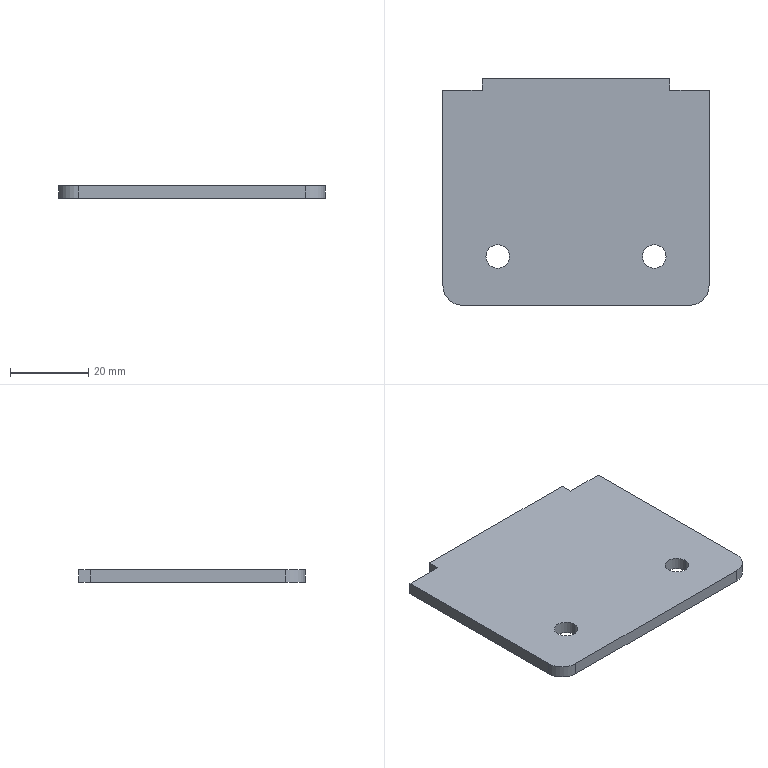Part | SolidWorks | features FlatPattern 1, SMBaseFlange 1, SheetMetal 1 | 1 solid | 16 faces | box 68 x 57.9 x 3.2 mm | volume 12192 mm3 | plane 10 | cylinder 6 | commonest cylinder face diameters 6 x4 10 x2
STEP:
#1=CARTESIAN_POINT('',(-23.,0.,3.2));
#2=VERTEX_POINT('',#1);
#3=CARTESIAN_POINT('',(-17.,0.,3.2));
#4=VERTEX_POINT('',#3);
#5=CARTESIAN_POINT('',(-20.,0.,3.2));
#6=DIRECTION('',(0.,0.,1.));
#7=DIRECTION('',(1.,0.,0.));
#8=AXIS2_PLACEMENT_3D('',#5,#6,#7);
#9=CIRCLE('',#8,3.);
#10=EDGE_CURVE('',#2,#4,#9,.T.);
#11=ORIENTED_EDGE('',*,*,#10,.T.);
#12=CARTESIAN_POINT('',(-17.,0.,0.));
#13=VERTEX_POINT('',#12);
#14=CARTESIAN_POINT('',(-17.,0.,3.2));
#15=DIRECTION('',(0.,0.,-1.));
#16=VECTOR('',#15,1000.);
#17=LINE('',#14,#16);
#18=EDGE_CURVE('',#4,#13,#17,.T.);
#19=ORIENTED_EDGE('',*,*,#18,.T.);
#20=CARTESIAN_POINT('',(-23.,0.,0.));
#21=VERTEX_POINT('',#20);
#22=CARTESIAN_POINT('',(-20.,0.,0.));
#23=DIRECTION('',(0.,0.,1.));
#24=DIRECTION('',(1.,0.,0.));
#25=AXIS2_PLACEMENT_3D('',#22,#23,#24);
#26=CIRCLE('',#25,3.);
#27=EDGE_CURVE('',#21,#13,#26,.T.);
#28=ORIENTED_EDGE('',*,*,#27,.F.);
#29=CARTESIAN_POINT('',(-23.,0.,3.2));
#30=DIRECTION('',(0.,0.,-1.));
#31=VECTOR('',#30,1000.);
#32=LINE('',#29,#31);
#33=EDGE_CURVE('',#2,#21,#32,.T.);
#34=ORIENTED_EDGE('',*,*,#33,.F.);
#35=EDGE_LOOP('',(#11,#19,#28,#34));
#36=FACE_OUTER_BOUND('',#35,.T.);
#37=CARTESIAN_POINT('',(-20.,0.,3.2));
#38=DIRECTION('',(0.,0.,-1.));
#39=DIRECTION('',(-1.,0.,0.));
#40=AXIS2_PLACEMENT_3D('',#37,#38,#39);
#41=CYLINDRICAL_SURFACE('',#40,3.);
#42=ADVANCED_FACE('',(#36),#41,.F.);
#43=CARTESIAN_POINT('',(17.,0.,3.2));
#44=VERTEX_POINT('',#43);
#45=CARTESIAN_POINT('',(23.,0.,3.2));
#46=VERTEX_POINT('',#45);
#47=CARTESIAN_POINT('',(20.,0.,3.2));
#48=DIRECTION('',(0.,0.,1.));
#49=DIRECTION('',(1.,0.,0.));
#50=AXIS2_PLACEMENT_3D('',#47,#48,#49);
#51=CIRCLE('',#50,3.);
#52=EDGE_CURVE('',#44,#46,#51,.T.);
#53=ORIENTED_EDGE('',*,*,#52,.T.);
#54=CARTESIAN_POINT('',(23.,0.,0.));
#55=VERTEX_POINT('',#54);
#56=CARTESIAN_POINT('',(23.,0.,3.2));
#57=DIRECTION('',(0.,0.,-1.));
#58=VECTOR('',#57,1000.);
#59=LINE('',#56,#58);
#60=EDGE_CURVE('',#46,#55,#59,.T.);
#61=ORIENTED_EDGE('',*,*,#60,.T.);
#62=CARTESIAN_POINT('',(17.,0.,0.));
#63=VERTEX_POINT('',#62);
#64=CARTESIAN_POINT('',(20.,0.,0.));
#65=DIRECTION('',(0.,0.,1.));
#66=DIRECTION('',(1.,0.,0.));
#67=AXIS2_PLACEMENT_3D('',#64,#65,#66);
#68=CIRCLE('',#67,3.);
#69=EDGE_CURVE('',#63,#55,#68,.T.);
#70=ORIENTED_EDGE('',*,*,#69,.F.);
#71=CARTESIAN_POINT('',(17.,0.,3.2));
#72=DIRECTION('',(0.,0.,-1.));
#73=VECTOR('',#72,1000.);
#74=LINE('',#71,#73);
#75=EDGE_CURVE('',#44,#63,#74,.T.);
#76=ORIENTED_EDGE('',*,*,#75,.F.);
#77=EDGE_LOOP('',(#53,#61,#70,#76));
#78=FACE_OUTER_BOUND('',#77,.T.);
#79=CARTESIAN_POINT('',(20.,0.,3.2));
#80=DIRECTION('',(0.,0.,-1.));
#81=DIRECTION('',(-1.,0.,0.));
#82=AXIS2_PLACEMENT_3D('',#79,#80,#81);
#83=CYLINDRICAL_SURFACE('',#82,3.);
#84=ADVANCED_FACE('',(#78),#83,.F.);
#85=CARTESIAN_POINT('',(34.,-7.5,3.2));
#86=VERTEX_POINT('',#85);
#87=CARTESIAN_POINT('',(34.,42.4,3.2));
#88=VERTEX_POINT('',#87);
#89=CARTESIAN_POINT('',(34.,0.,3.2));
#90=DIRECTION('',(0.,1.,0.));
#91=VECTOR('',#90,1000.);
#92=LINE('',#89,#91);
#93=EDGE_CURVE('',#86,#88,#92,.T.);
#94=ORIENTED_EDGE('',*,*,#93,.T.);
#95=CARTESIAN_POINT('',(24.,42.4,3.2));
#96=VERTEX_POINT('',#95);
#97=CARTESIAN_POINT('',(34.,42.4,3.2));
#98=DIRECTION('',(-1.,0.,0.));
#99=VECTOR('',#98,1000.);
#100=LINE('',#97,#99);
#101=EDGE_CURVE('',#88,#96,#100,.T.);
#102=ORIENTED_EDGE('',*,*,#101,.T.);
#103=CARTESIAN_POINT('',(24.,45.4,3.2));
#104=VERTEX_POINT('',#103);
#105=CARTESIAN_POINT('',(24.,42.4,3.2));
#106=DIRECTION('',(0.,1.,0.));
#107=VECTOR('',#106,1000.);
#108=LINE('',#105,#107);
#109=EDGE_CURVE('',#96,#104,#108,.T.);
#110=ORIENTED_EDGE('',*,*,#109,.T.);
#111=CARTESIAN_POINT('',(-24.,45.4,3.2));
#112=VERTEX_POINT('',#111);
#113=CARTESIAN_POINT('',(24.,45.4,3.2));
#114=DIRECTION('',(-1.,0.,0.));
#115=VECTOR('',#114,1000.);
#116=LINE('',#113,#115);
#117=EDGE_CURVE('',#104,#112,#116,.T.);
#118=ORIENTED_EDGE('',*,*,#117,.T.);
#119=CARTESIAN_POINT('',(-24.,42.4,3.2));
#120=VERTEX_POINT('',#119);
#121=CARTESIAN_POINT('',(-24.,45.4,3.2));
#122=DIRECTION('',(0.,-1.,0.));
#123=VECTOR('',#122,1000.);
#124=LINE('',#121,#123);
#125=EDGE_CURVE('',#112,#120,#124,.T.);
#126=ORIENTED_EDGE('',*,*,#125,.T.);
#127=CARTESIAN_POINT('',(-34.,42.4,3.2));
#128=VERTEX_POINT('',#127);
#129=CARTESIAN_POINT('',(-24.,42.4,3.2));
#130=DIRECTION('',(-1.,0.,0.));
#131=VECTOR('',#130,1000.);
#132=LINE('',#129,#131);
#133=EDGE_CURVE('',#120,#128,#132,.T.);
#134=ORIENTED_EDGE('',*,*,#133,.T.);
#135=CARTESIAN_POINT('',(-34.,-7.5,3.2));
#136=VERTEX_POINT('',#135);
#137=CARTESIAN_POINT('',(-34.,42.4,3.2));
#138=DIRECTION('',(0.,-1.,0.));
#139=VECTOR('',#138,1000.);
#140=LINE('',#137,#139);
#141=EDGE_CURVE('',#128,#136,#140,.T.);
#142=ORIENTED_EDGE('',*,*,#141,.T.);
#143=CARTESIAN_POINT('',(-29.,-12.5,3.2));
#144=VERTEX_POINT('',#143);
#145=CARTESIAN_POINT('',(-29.,-7.5,3.2));
#146=DIRECTION('',(0.,0.,1.));
#147=DIRECTION('',(-1.,0.,0.));
#148=AXIS2_PLACEMENT_3D('',#145,#146,#147);
#149=CIRCLE('',#148,5.);
#150=EDGE_CURVE('',#136,#144,#149,.T.);
#151=ORIENTED_EDGE('',*,*,#150,.T.);
#152=CARTESIAN_POINT('',(29.,-12.5,3.2));
#153=VERTEX_POINT('',#152);
#154=CARTESIAN_POINT('',(29.,-12.5,3.2));
#155=DIRECTION('',(1.,0.,0.));
#156=VECTOR('',#155,1000.);
#157=LINE('',#154,#156);
#158=EDGE_CURVE('',#144,#153,#157,.T.);
#159=ORIENTED_EDGE('',*,*,#158,.T.);
#160=CARTESIAN_POINT('',(29.,-7.5,3.2));
#161=DIRECTION('',(0.,0.,1.));
#162=DIRECTION('',(-1.,0.,0.));
#163=AXIS2_PLACEMENT_3D('',#160,#161,#162);
#164=CIRCLE('',#163,5.);
#165=EDGE_CURVE('',#153,#86,#164,.T.);
#166=ORIENTED_EDGE('',*,*,#165,.T.);
#167=EDGE_LOOP('',(#94,#102,#110,#118,#126,#134,#142,#151,#159,#166));
#168=FACE_OUTER_BOUND('',#167,.T.);
#169=ORIENTED_EDGE('',*,*,#52,.F.);
#170=CARTESIAN_POINT('',(20.,0.,3.2));
#171=DIRECTION('',(0.,0.,1.));
#172=DIRECTION('',(1.,0.,0.));
#173=AXIS2_PLACEMENT_3D('',#170,#171,#172);
#174=CIRCLE('',#173,3.);
#175=EDGE_CURVE('',#46,#44,#174,.T.);
#176=ORIENTED_EDGE('',*,*,#175,.F.);
#177=EDGE_LOOP('',(#169,#176));
#178=FACE_BOUND('',#177,.T.);
#179=ORIENTED_EDGE('',*,*,#10,.F.);
#180=CARTESIAN_POINT('',(-20.,0.,3.2));
#181=DIRECTION('',(0.,0.,1.));
#182=DIRECTION('',(1.,0.,0.));
#183=AXIS2_PLACEMENT_3D('',#180,#181,#182);
#184=CIRCLE('',#183,3.);
#185=EDGE_CURVE('',#4,#2,#184,.T.);
#186=ORIENTED_EDGE('',*,*,#185,.F.);
#187=EDGE_LOOP('',(#179,#186));
#188=FACE_BOUND('',#187,.T.);
#189=CARTESIAN_POINT('',(29.,-7.5,3.2));
#190=DIRECTION('',(0.,0.,-1.));
#191=DIRECTION('',(-1.,0.,0.));
#192=AXIS2_PLACEMENT_3D('',#189,#190,#191);
#193=PLANE('',#192);
#194=ADVANCED_FACE('',(#168,#178,#188),#193,.F.);
#195=ORIENTED_EDGE('',*,*,#69,.T.);
#196=CARTESIAN_POINT('',(20.,0.,0.));
#197=DIRECTION('',(0.,0.,1.));
#198=DIRECTION('',(1.,0.,0.));
#199=AXIS2_PLACEMENT_3D('',#196,#197,#198);
#200=CIRCLE('',#199,3.);
#201=EDGE_CURVE('',#55,#63,#200,.T.);
#202=ORIENTED_EDGE('',*,*,#201,.T.);
#203=EDGE_LOOP('',(#195,#202));
#204=FACE_BOUND('',#203,.T.);
#205=CARTESIAN_POINT('',(34.,-7.5,0.));
#206=VERTEX_POINT('',#205);
#207=CARTESIAN_POINT('',(34.,42.4,0.));
#208=VERTEX_POINT('',#207);
#209=CARTESIAN_POINT('',(34.,0.,0.));
#210=DIRECTION('',(0.,1.,0.));
#211=VECTOR('',#210,1000.);
#212=LINE('',#209,#211);
#213=EDGE_CURVE('',#206,#208,#212,.T.);
#214=ORIENTED_EDGE('',*,*,#213,.F.);
#215=CARTESIAN_POINT('',(29.,-12.5,0.));
#216=VERTEX_POINT('',#215);
#217=CARTESIAN_POINT('',(29.,-7.5,0.));
#218=DIRECTION('',(0.,0.,1.));
#219=DIRECTION('',(-1.,0.,0.));
#220=AXIS2_PLACEMENT_3D('',#217,#218,#219);
#221=CIRCLE('',#220,5.);
#222=EDGE_CURVE('',#216,#206,#221,.T.);
#223=ORIENTED_EDGE('',*,*,#222,.F.);
#224=CARTESIAN_POINT('',(-29.,-12.5,0.));
#225=VERTEX_POINT('',#224);
#226=CARTESIAN_POINT('',(29.,-12.5,0.));
#227=DIRECTION('',(1.,0.,0.));
#228=VECTOR('',#227,1000.);
#229=LINE('',#226,#228);
#230=EDGE_CURVE('',#225,#216,#229,.T.);
#231=ORIENTED_EDGE('',*,*,#230,.F.);
#232=CARTESIAN_POINT('',(-34.,-7.5,0.));
#233=VERTEX_POINT('',#232);
#234=CARTESIAN_POINT('',(-29.,-7.5,0.));
#235=DIRECTION('',(0.,0.,1.));
#236=DIRECTION('',(-1.,0.,0.));
#237=AXIS2_PLACEMENT_3D('',#234,#235,#236);
#238=CIRCLE('',#237,5.);
#239=EDGE_CURVE('',#233,#225,#238,.T.);
#240=ORIENTED_EDGE('',*,*,#239,.F.);
#241=CARTESIAN_POINT('',(-34.,42.4,0.));
#242=VERTEX_POINT('',#241);
#243=CARTESIAN_POINT('',(-34.,-7.5,0.));
#244=DIRECTION('',(0.,-1.,0.));
#245=VECTOR('',#244,1000.);
#246=LINE('',#243,#245);
#247=EDGE_CURVE('',#242,#233,#246,.T.);
#248=ORIENTED_EDGE('',*,*,#247,.F.);
#249=CARTESIAN_POINT('',(-24.,42.4,0.));
#250=VERTEX_POINT('',#249);
#251=CARTESIAN_POINT('',(-24.,42.4,0.));
#252=DIRECTION('',(-1.,0.,0.));
#253=VECTOR('',#252,1000.);
#254=LINE('',#251,#253);
#255=EDGE_CURVE('',#250,#242,#254,.T.);
#256=ORIENTED_EDGE('',*,*,#255,.F.);
#257=CARTESIAN_POINT('',(-24.,45.4,0.));
#258=VERTEX_POINT('',#257);
#259=CARTESIAN_POINT('',(-24.,45.4,0.));
#260=DIRECTION('',(0.,-1.,0.));
#261=VECTOR('',#260,1000.);
#262=LINE('',#259,#261);
#263=EDGE_CURVE('',#258,#250,#262,.T.);
#264=ORIENTED_EDGE('',*,*,#263,.F.);
#265=CARTESIAN_POINT('',(24.,45.4,0.));
#266=VERTEX_POINT('',#265);
#267=CARTESIAN_POINT('',(24.,45.4,0.));
#268=DIRECTION('',(-1.,0.,0.));
#269=VECTOR('',#268,1000.);
#270=LINE('',#267,#269);
#271=EDGE_CURVE('',#266,#258,#270,.T.);
#272=ORIENTED_EDGE('',*,*,#271,.F.);
#273=CARTESIAN_POINT('',(24.,42.4,0.));
#274=VERTEX_POINT('',#273);
#275=CARTESIAN_POINT('',(24.,42.4,0.));
#276=DIRECTION('',(0.,1.,0.));
#277=VECTOR('',#276,1000.);
#278=LINE('',#275,#277);
#279=EDGE_CURVE('',#274,#266,#278,.T.);
#280=ORIENTED_EDGE('',*,*,#279,.F.);
#281=CARTESIAN_POINT('',(34.,42.4,0.));
#282=DIRECTION('',(-1.,0.,0.));
#283=VECTOR('',#282,1000.);
#284=LINE('',#281,#283);
#285=EDGE_CURVE('',#208,#274,#284,.T.);
#286=ORIENTED_EDGE('',*,*,#285,.F.);
#287=EDGE_LOOP('',(#214,#223,#231,#240,#248,#256,#264,#272,#280,#286));
#288=FACE_OUTER_BOUND('',#287,.T.);
#289=ORIENTED_EDGE('',*,*,#27,.T.);
#290=CARTESIAN_POINT('',(-20.,0.,0.));
#291=DIRECTION('',(0.,0.,1.));
#292=DIRECTION('',(1.,0.,0.));
#293=AXIS2_PLACEMENT_3D('',#290,#291,#292);
#294=CIRCLE('',#293,3.);
#295=EDGE_CURVE('',#13,#21,#294,.T.);
#296=ORIENTED_EDGE('',*,*,#295,.T.);
#297=EDGE_LOOP('',(#289,#296));
#298=FACE_BOUND('',#297,.T.);
#299=CARTESIAN_POINT('',(29.,-7.5,0.));
#300=DIRECTION('',(0.,0.,-1.));
#301=DIRECTION('',(-1.,0.,0.));
#302=AXIS2_PLACEMENT_3D('',#299,#300,#301);
#303=PLANE('',#302);
#304=ADVANCED_FACE('',(#204,#288,#298),#303,.T.);
#305=ORIENTED_EDGE('',*,*,#213,.T.);
#306=CARTESIAN_POINT('',(34.,42.4,3.2));
#307=DIRECTION('',(0.,0.,-1.));
#308=VECTOR('',#307,1000.);
#309=LINE('',#306,#308);
#310=EDGE_CURVE('',#88,#208,#309,.T.);
#311=ORIENTED_EDGE('',*,*,#310,.F.);
#312=ORIENTED_EDGE('',*,*,#93,.F.);
#313=CARTESIAN_POINT('',(34.,-7.5,3.2));
#314=DIRECTION('',(0.,0.,-1.));
#315=VECTOR('',#314,1000.);
#316=LINE('',#313,#315);
#317=EDGE_CURVE('',#86,#206,#316,.T.);
#318=ORIENTED_EDGE('',*,*,#317,.T.);
#319=EDGE_LOOP('',(#305,#311,#312,#318));
#320=FACE_OUTER_BOUND('',#319,.T.);
#321=CARTESIAN_POINT('',(34.,0.,3.2));
#322=DIRECTION('',(-1.,0.,0.));
#323=DIRECTION('',(0.,0.,1.));
#324=AXIS2_PLACEMENT_3D('',#321,#322,#323);
#325=PLANE('',#324);
#326=ADVANCED_FACE('',(#320),#325,.F.);
#327=ORIENTED_EDGE('',*,*,#285,.T.);
#328=CARTESIAN_POINT('',(24.,42.4,3.2));
#329=DIRECTION('',(0.,0.,-1.));
#330=VECTOR('',#329,1000.);
#331=LINE('',#328,#330);
#332=EDGE_CURVE('',#96,#274,#331,.T.);
#333=ORIENTED_EDGE('',*,*,#332,.F.);
#334=ORIENTED_EDGE('',*,*,#101,.F.);
#335=ORIENTED_EDGE('',*,*,#310,.T.);
#336=EDGE_LOOP('',(#327,#333,#334,#335));
#337=FACE_OUTER_BOUND('',#336,.T.);
#338=CARTESIAN_POINT('',(34.,42.4,3.2));
#339=DIRECTION('',(0.,-1.,0.));
#340=DIRECTION('',(0.,0.,-1.));
#341=AXIS2_PLACEMENT_3D('',#338,#339,#340);
#342=PLANE('',#341);
#343=ADVANCED_FACE('',(#337),#342,.F.);
#344=ORIENTED_EDGE('',*,*,#279,.T.);
#345=CARTESIAN_POINT('',(24.,45.4,3.2));
#346=DIRECTION('',(0.,0.,-1.));
#347=VECTOR('',#346,1000.);
#348=LINE('',#345,#347);
#349=EDGE_CURVE('',#104,#266,#348,.T.);
#350=ORIENTED_EDGE('',*,*,#349,.F.);
#351=ORIENTED_EDGE('',*,*,#109,.F.);
#352=ORIENTED_EDGE('',*,*,#332,.T.);
#353=EDGE_LOOP('',(#344,#350,#351,#352));
#354=FACE_OUTER_BOUND('',#353,.T.);
#355=CARTESIAN_POINT('',(24.,42.4,3.2));
#356=DIRECTION('',(-1.,0.,0.));
#357=DIRECTION('',(0.,0.,1.));
#358=AXIS2_PLACEMENT_3D('',#355,#356,#357);
#359=PLANE('',#358);
#360=ADVANCED_FACE('',(#354),#359,.F.);
#361=ORIENTED_EDGE('',*,*,#271,.T.);
#362=CARTESIAN_POINT('',(-24.,45.4,3.2));
#363=DIRECTION('',(0.,0.,-1.));
#364=VECTOR('',#363,1000.);
#365=LINE('',#362,#364);
#366=EDGE_CURVE('',#112,#258,#365,.T.);
#367=ORIENTED_EDGE('',*,*,#366,.F.);
#368=ORIENTED_EDGE('',*,*,#117,.F.);
#369=ORIENTED_EDGE('',*,*,#349,.T.);
#370=EDGE_LOOP('',(#361,#367,#368,#369));
#371=FACE_OUTER_BOUND('',#370,.T.);
#372=CARTESIAN_POINT('',(24.,45.4,3.2));
#373=DIRECTION('',(0.,-1.,0.));
#374=DIRECTION('',(1.,0.,0.));
#375=AXIS2_PLACEMENT_3D('',#372,#373,#374);
#376=PLANE('',#375);
#377=ADVANCED_FACE('',(#371),#376,.F.);
#378=ORIENTED_EDGE('',*,*,#263,.T.);
#379=CARTESIAN_POINT('',(-24.,42.4,3.2));
#380=DIRECTION('',(0.,0.,-1.));
#381=VECTOR('',#380,1000.);
#382=LINE('',#379,#381);
#383=EDGE_CURVE('',#120,#250,#382,.T.);
#384=ORIENTED_EDGE('',*,*,#383,.F.);
#385=ORIENTED_EDGE('',*,*,#125,.F.);
#386=ORIENTED_EDGE('',*,*,#366,.T.);
#387=EDGE_LOOP('',(#378,#384,#385,#386));
#388=FACE_OUTER_BOUND('',#387,.T.);
#389=CARTESIAN_POINT('',(-24.,45.4,3.2));
#390=DIRECTION('',(1.,0.,0.));
#391=DIRECTION('',(0.,0.,-1.));
#392=AXIS2_PLACEMENT_3D('',#389,#390,#391);
#393=PLANE('',#392);
#394=ADVANCED_FACE('',(#388),#393,.F.);
#395=ORIENTED_EDGE('',*,*,#255,.T.);
#396=CARTESIAN_POINT('',(-34.,42.4,3.2));
#397=DIRECTION('',(0.,0.,-1.));
#398=VECTOR('',#397,1000.);
#399=LINE('',#396,#398);
#400=EDGE_CURVE('',#128,#242,#399,.T.);
#401=ORIENTED_EDGE('',*,*,#400,.F.);
#402=ORIENTED_EDGE('',*,*,#133,.F.);
#403=ORIENTED_EDGE('',*,*,#383,.T.);
#404=EDGE_LOOP('',(#395,#401,#402,#403));
#405=FACE_OUTER_BOUND('',#404,.T.);
#406=CARTESIAN_POINT('',(-24.,42.4,3.2));
#407=DIRECTION('',(0.,-1.,0.));
#408=DIRECTION('',(1.,0.,0.));
#409=AXIS2_PLACEMENT_3D('',#406,#407,#408);
#410=PLANE('',#409);
#411=ADVANCED_FACE('',(#405),#410,.F.);
#412=ORIENTED_EDGE('',*,*,#247,.T.);
#413=CARTESIAN_POINT('',(-34.,-7.5,3.2));
#414=DIRECTION('',(0.,0.,-1.));
#415=VECTOR('',#414,1000.);
#416=LINE('',#413,#415);
#417=EDGE_CURVE('',#136,#233,#416,.T.);
#418=ORIENTED_EDGE('',*,*,#417,.F.);
#419=ORIENTED_EDGE('',*,*,#141,.F.);
#420=ORIENTED_EDGE('',*,*,#400,.T.);
#421=EDGE_LOOP('',(#412,#418,#419,#420));
#422=FACE_OUTER_BOUND('',#421,.T.);
#423=CARTESIAN_POINT('',(-34.,-7.5,3.2));
#424=DIRECTION('',(1.,0.,0.));
#425=DIRECTION('',(0.,1.,0.));
#426=AXIS2_PLACEMENT_3D('',#423,#424,#425);
#427=PLANE('',#426);
#428=ADVANCED_FACE('',(#422),#427,.F.);
#429=ORIENTED_EDGE('',*,*,#239,.T.);
#430=CARTESIAN_POINT('',(-29.,-12.5,3.2));
#431=DIRECTION('',(0.,0.,-1.));
#432=VECTOR('',#431,1000.);
#433=LINE('',#430,#432);
#434=EDGE_CURVE('',#144,#225,#433,.T.);
#435=ORIENTED_EDGE('',*,*,#434,.F.);
#436=ORIENTED_EDGE('',*,*,#150,.F.);
#437=ORIENTED_EDGE('',*,*,#417,.T.);
#438=EDGE_LOOP('',(#429,#435,#436,#437));
#439=FACE_OUTER_BOUND('',#438,.T.);
#440=CARTESIAN_POINT('',(-29.,-7.5,3.2));
#441=DIRECTION('',(0.,0.,-1.));
#442=DIRECTION('',(-1.,0.,0.));
#443=AXIS2_PLACEMENT_3D('',#440,#441,#442);
#444=CYLINDRICAL_SURFACE('',#443,5.);
#445=ADVANCED_FACE('',(#439),#444,.T.);
#446=ORIENTED_EDGE('',*,*,#230,.T.);
#447=CARTESIAN_POINT('',(29.,-12.5,3.2));
#448=DIRECTION('',(0.,0.,-1.));
#449=VECTOR('',#448,1000.);
#450=LINE('',#447,#449);
#451=EDGE_CURVE('',#153,#216,#450,.T.);
#452=ORIENTED_EDGE('',*,*,#451,.F.);
#453=ORIENTED_EDGE('',*,*,#158,.F.);
#454=ORIENTED_EDGE('',*,*,#434,.T.);
#455=EDGE_LOOP('',(#446,#452,#453,#454));
#456=FACE_OUTER_BOUND('',#455,.T.);
#457=CARTESIAN_POINT('',(29.,-12.5,3.2));
#458=DIRECTION('',(0.,1.,0.));
#459=DIRECTION('',(-1.,0.,0.));
#460=AXIS2_PLACEMENT_3D('',#457,#458,#459);
#461=PLANE('',#460);
#462=ADVANCED_FACE('',(#456),#461,.F.);
#463=ORIENTED_EDGE('',*,*,#222,.T.);
#464=ORIENTED_EDGE('',*,*,#317,.F.);
#465=ORIENTED_EDGE('',*,*,#165,.F.);
#466=ORIENTED_EDGE('',*,*,#451,.T.);
#467=EDGE_LOOP('',(#463,#464,#465,#466));
#468=FACE_OUTER_BOUND('',#467,.T.);
#469=CARTESIAN_POINT('',(29.,-7.5,3.2));
#470=DIRECTION('',(0.,0.,-1.));
#471=DIRECTION('',(-1.,0.,0.));
#472=AXIS2_PLACEMENT_3D('',#469,#470,#471);
#473=CYLINDRICAL_SURFACE('',#472,5.);
#474=ADVANCED_FACE('',(#468),#473,.T.);
#475=ORIENTED_EDGE('',*,*,#60,.F.);
#476=ORIENTED_EDGE('',*,*,#175,.T.);
#477=ORIENTED_EDGE('',*,*,#75,.T.);
#478=ORIENTED_EDGE('',*,*,#201,.F.);
#479=EDGE_LOOP('',(#475,#476,#477,#478));
#480=FACE_OUTER_BOUND('',#479,.T.);
#481=CARTESIAN_POINT('',(20.,0.,3.2));
#482=DIRECTION('',(0.,0.,-1.));
#483=DIRECTION('',(-1.,0.,0.));
#484=AXIS2_PLACEMENT_3D('',#481,#482,#483);
#485=CYLINDRICAL_SURFACE('',#484,3.);
#486=ADVANCED_FACE('',(#480),#485,.F.);
#487=ORIENTED_EDGE('',*,*,#18,.F.);
#488=ORIENTED_EDGE('',*,*,#185,.T.);
#489=ORIENTED_EDGE('',*,*,#33,.T.);
#490=ORIENTED_EDGE('',*,*,#295,.F.);
#491=EDGE_LOOP('',(#487,#488,#489,#490));
#492=FACE_OUTER_BOUND('',#491,.T.);
#493=CARTESIAN_POINT('',(-20.,0.,3.2));
#494=DIRECTION('',(0.,0.,-1.));
#495=DIRECTION('',(-1.,0.,0.));
#496=AXIS2_PLACEMENT_3D('',#493,#494,#495);
#497=CYLINDRICAL_SURFACE('',#496,3.);
#498=ADVANCED_FACE('',(#492),#497,.F.);
#499=CLOSED_SHELL('',(#42,#84,#194,#304,#326,#343,#360,#377,#394,#411,#428,#445,#462,#474,#486,#498));
#500=MANIFOLD_SOLID_BREP('',#499);
#501=CARTESIAN_POINT('',(0.,0.,0.));
#502=DIRECTION('',(0.,0.,1.));
#503=DIRECTION('',(1.,0.,0.));
#504=AXIS2_PLACEMENT_3D('',#501,#502,#503);
#505=(LENGTH_UNIT()NAMED_UNIT(*)SI_UNIT(.MILLI.,.METRE.));
#506=UNCERTAINTY_MEASURE_WITH_UNIT(LENGTH_MEASURE(0.00001),#505,'','');
#507=(NAMED_UNIT(*)PLANE_ANGLE_UNIT()SI_UNIT($,.RADIAN.));
#508=(NAMED_UNIT(*)SI_UNIT($,.STERADIAN.)SOLID_ANGLE_UNIT());
#509=(GEOMETRIC_REPRESENTATION_CONTEXT(3)GLOBAL_UNCERTAINTY_ASSIGNED_CONTEXT((#506))GLOBAL_UNIT_ASSIGNED_CONTEXT((#505,#507,#508))REPRESENTATION_CONTEXT('',''));
#510=ADVANCED_BREP_SHAPE_REPRESENTATION('',(#500,#504),#509);